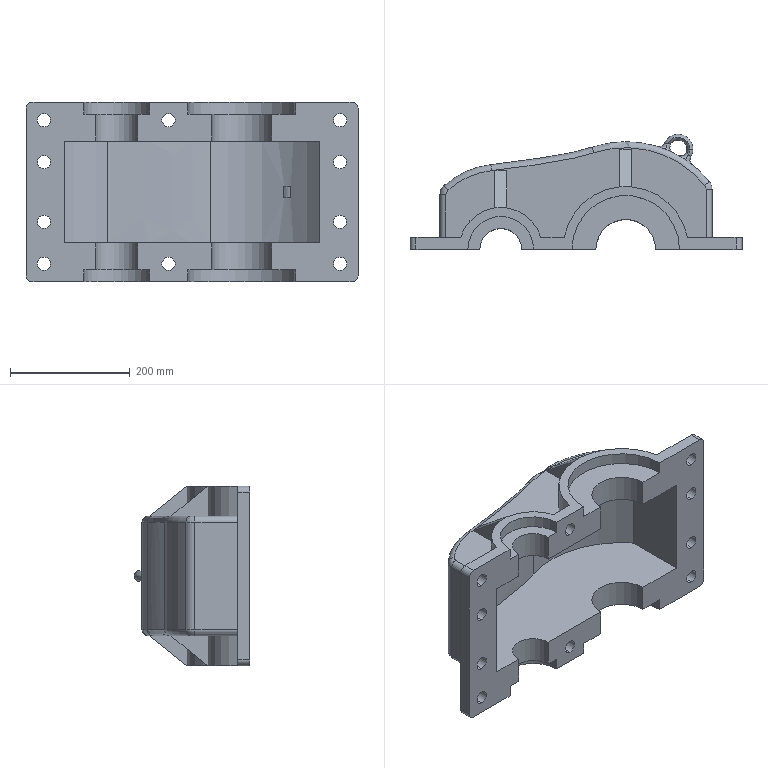Part | SolidWorks | features ICE 8, Fillet 4, Extrusion 1, MirrorPattern 1, Shell 1 | 1 solid | 117 faces | box 555 x 192.629 x 300 mm | volume 5936762 mm3 | cylinder 51 | plane 38 | torus 16 | spline 12 | commonest cylinder face diameters 22 x20 20 x8 140 x4 210 x4 40 x2 70 x2